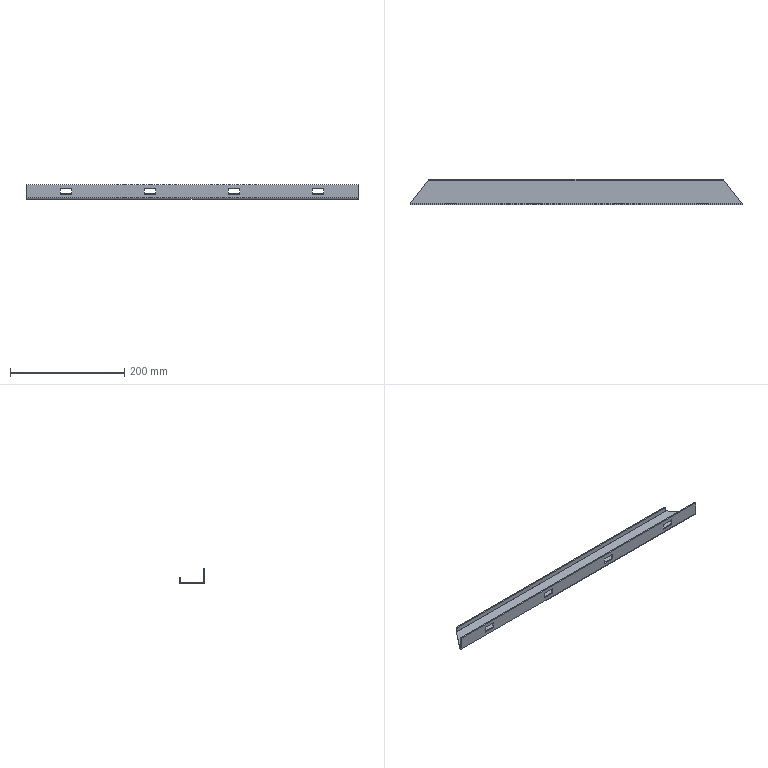Part | STEP file | Right Door Frame 4 | 1 solid | 36 faces | box 580 x 45 x 25 mm | volume 81646 mm3 | plane 32 | cylinder 4 | commonest cylinder face diameters 0.2 x2 4.2 x2
STEP:
#1=CARTESIAN_POINT('',(480.95,42.998,-6.375));
#2=VERTEX_POINT('',#1);
#3=CARTESIAN_POINT('',(480.95,43.,-6.375));
#4=VERTEX_POINT('',#3);
#5=CARTESIAN_POINT('',(480.95,40.9,-6.375));
#6=DIRECTION('',(0.,1.,0.));
#7=VECTOR('',#6,1000.);
#8=LINE('',#5,#7);
#9=EDGE_CURVE('',#2,#4,#8,.T.);
#10=ORIENTED_EDGE('',*,*,#9,.F.);
#11=CARTESIAN_POINT('',(480.95,40.9,-6.375));
#12=VERTEX_POINT('',#11);
#13=CARTESIAN_POINT('',(480.95,0.,-6.375));
#14=DIRECTION('',(0.,-1.,0.));
#15=VECTOR('',#14,1000.);
#16=LINE('',#13,#15);
#17=EDGE_CURVE('',#2,#12,#16,.T.);
#18=ORIENTED_EDGE('',*,*,#17,.T.);
#19=CARTESIAN_POINT('',(-33.05,40.9,-6.375));
#20=VERTEX_POINT('',#19);
#21=CARTESIAN_POINT('',(0.,40.9,-6.375));
#22=DIRECTION('',(-1.,0.,0.));
#23=VECTOR('',#22,1000.);
#24=LINE('',#21,#23);
#25=EDGE_CURVE('',#12,#20,#24,.T.);
#26=ORIENTED_EDGE('',*,*,#25,.T.);
#27=CARTESIAN_POINT('',(-33.05,42.998,-6.375));
#28=VERTEX_POINT('',#27);
#29=CARTESIAN_POINT('',(-33.05,0.,-6.375));
#30=DIRECTION('',(0.,1.,0.));
#31=VECTOR('',#30,1000.);
#32=LINE('',#29,#31);
#33=EDGE_CURVE('',#20,#28,#32,.T.);
#34=ORIENTED_EDGE('',*,*,#33,.T.);
#35=CARTESIAN_POINT('',(-33.05,43.,-6.375));
#36=VERTEX_POINT('',#35);
#37=CARTESIAN_POINT('',(-33.05,43.,-6.375));
#38=DIRECTION('',(0.,-1.,0.));
#39=VECTOR('',#38,1000.);
#40=LINE('',#37,#39);
#41=EDGE_CURVE('',#36,#28,#40,.T.);
#42=ORIENTED_EDGE('',*,*,#41,.F.);
#43=CARTESIAN_POINT('',(-66.05,0.2,-6.375));
#44=VERTEX_POINT('',#43);
#45=CARTESIAN_POINT('',(-33.05,43.,-6.375));
#46=DIRECTION('',(-0.6106,-0.7919,0.));
#47=VECTOR('',#46,1000.);
#48=LINE('',#45,#47);
#49=EDGE_CURVE('',#36,#44,#48,.T.);
#50=ORIENTED_EDGE('',*,*,#49,.T.);
#51=CARTESIAN_POINT('',(-66.05,0.1,-6.375));
#52=VERTEX_POINT('',#51);
#53=CARTESIAN_POINT('',(-66.05,43.,-6.375));
#54=DIRECTION('',(0.,-1.,0.));
#55=VECTOR('',#54,1000.);
#56=LINE('',#53,#55);
#57=EDGE_CURVE('',#44,#52,#56,.T.);
#58=ORIENTED_EDGE('',*,*,#57,.T.);
#59=CARTESIAN_POINT('',(513.95,0.1,-6.375));
#60=VERTEX_POINT('',#59);
#61=CARTESIAN_POINT('',(0.,0.1,-6.375));
#62=DIRECTION('',(1.,0.,0.));
#63=VECTOR('',#62,1000.);
#64=LINE('',#61,#63);
#65=EDGE_CURVE('',#52,#60,#64,.T.);
#66=ORIENTED_EDGE('',*,*,#65,.T.);
#67=CARTESIAN_POINT('',(513.95,0.2,-6.375));
#68=VERTEX_POINT('',#67);
#69=CARTESIAN_POINT('',(513.95,0.,-6.375));
#70=DIRECTION('',(0.,1.,0.));
#71=VECTOR('',#70,1000.);
#72=LINE('',#69,#71);
#73=EDGE_CURVE('',#60,#68,#72,.T.);
#74=ORIENTED_EDGE('',*,*,#73,.T.);
#75=CARTESIAN_POINT('',(513.95,0.2,-6.375));
#76=DIRECTION('',(-0.6106,0.7919,0.));
#77=VECTOR('',#76,1000.);
#78=LINE('',#75,#77);
#79=EDGE_CURVE('',#68,#4,#78,.T.);
#80=ORIENTED_EDGE('',*,*,#79,.T.);
#81=EDGE_LOOP('',(#10,#18,#26,#34,#42,#50,#58,#66,#74,#80));
#82=FACE_OUTER_BOUND('',#81,.T.);
#83=CARTESIAN_POINT('',(0.,0.,-6.375));
#84=DIRECTION('',(0.,0.,1.));
#85=DIRECTION('',(0.,-1.,0.));
#86=AXIS2_PLACEMENT_3D('',#83,#84,#85);
#87=PLANE('',#86);
#88=ADVANCED_FACE('',(#82),#87,.T.);
#89=CARTESIAN_POINT('',(480.95,43.,-6.275));
#90=VERTEX_POINT('',#89);
#91=CARTESIAN_POINT('',(480.95,40.9,-6.275));
#92=DIRECTION('',(-1.,0.,0.));
#93=DIRECTION('',(0.,0.,1.));
#94=AXIS2_PLACEMENT_3D('',#91,#92,#93);
#95=CIRCLE('',#94,2.1);
#96=EDGE_CURVE('',#90,#2,#95,.T.);
#97=ORIENTED_EDGE('',*,*,#96,.F.);
#98=CARTESIAN_POINT('',(480.95,43.,1.625));
#99=VERTEX_POINT('',#98);
#100=CARTESIAN_POINT('',(480.95,43.,-6.375));
#101=DIRECTION('',(0.,0.,-1.));
#102=VECTOR('',#101,1000.);
#103=LINE('',#100,#102);
#104=EDGE_CURVE('',#99,#90,#103,.T.);
#105=ORIENTED_EDGE('',*,*,#104,.F.);
#106=CARTESIAN_POINT('',(480.95,41.,1.625));
#107=VERTEX_POINT('',#106);
#108=CARTESIAN_POINT('',(480.95,43.,1.625));
#109=DIRECTION('',(0.,1.,0.));
#110=VECTOR('',#109,1000.);
#111=LINE('',#108,#110);
#112=EDGE_CURVE('',#107,#99,#111,.T.);
#113=ORIENTED_EDGE('',*,*,#112,.F.);
#114=CARTESIAN_POINT('',(480.95,41.,-6.275));
#115=VERTEX_POINT('',#114);
#116=CARTESIAN_POINT('',(480.95,41.,-6.375));
#117=DIRECTION('',(0.,0.,1.));
#118=VECTOR('',#117,1000.);
#119=LINE('',#116,#118);
#120=EDGE_CURVE('',#115,#107,#119,.T.);
#121=ORIENTED_EDGE('',*,*,#120,.F.);
#122=CARTESIAN_POINT('',(480.95,40.9,-6.275));
#123=DIRECTION('',(-1.,0.,0.));
#124=DIRECTION('',(0.,0.,1.));
#125=AXIS2_PLACEMENT_3D('',#122,#123,#124);
#126=CIRCLE('',#125,0.1);
#127=EDGE_CURVE('',#115,#12,#126,.T.);
#128=ORIENTED_EDGE('',*,*,#127,.T.);
#129=ORIENTED_EDGE('',*,*,#17,.F.);
#130=EDGE_LOOP('',(#97,#105,#113,#121,#128,#129));
#131=FACE_OUTER_BOUND('',#130,.T.);
#132=CARTESIAN_POINT('',(480.95,40.9,-6.275));
#133=DIRECTION('',(1.,0.,0.));
#134=DIRECTION('',(0.,0.,-1.));
#135=AXIS2_PLACEMENT_3D('',#132,#133,#134);
#136=PLANE('',#135);
#137=ADVANCED_FACE('',(#131),#136,.T.);
#138=CARTESIAN_POINT('',(513.95,0.2,-8.375));
#139=VERTEX_POINT('',#138);
#140=CARTESIAN_POINT('',(513.95,0.2,1.625));
#141=DIRECTION('',(0.,0.,1.));
#142=VECTOR('',#141,1000.);
#143=LINE('',#140,#142);
#144=EDGE_CURVE('',#139,#68,#143,.T.);
#145=ORIENTED_EDGE('',*,*,#144,.F.);
#146=CARTESIAN_POINT('',(480.95,43.,-8.375));
#147=VERTEX_POINT('',#146);
#148=CARTESIAN_POINT('',(513.95,0.2,-8.375));
#149=DIRECTION('',(0.6106,-0.7919,0.));
#150=VECTOR('',#149,1000.);
#151=LINE('',#148,#150);
#152=EDGE_CURVE('',#147,#139,#151,.T.);
#153=ORIENTED_EDGE('',*,*,#152,.F.);
#154=CARTESIAN_POINT('',(480.95,43.,1.625));
#155=DIRECTION('',(0.,0.,-1.));
#156=VECTOR('',#155,1000.);
#157=LINE('',#154,#156);
#158=EDGE_CURVE('',#4,#147,#157,.T.);
#159=ORIENTED_EDGE('',*,*,#158,.F.);
#160=ORIENTED_EDGE('',*,*,#79,.F.);
#161=EDGE_LOOP('',(#145,#153,#159,#160));
#162=FACE_OUTER_BOUND('',#161,.T.);
#163=CARTESIAN_POINT('',(513.95,0.2,1.625));
#164=DIRECTION('',(-0.7919,-0.6106,0.));
#165=DIRECTION('',(0.6106,-0.7919,0.));
#166=AXIS2_PLACEMENT_3D('',#163,#164,#165);
#167=PLANE('',#166);
#168=ADVANCED_FACE('',(#162),#167,.F.);
#169=CARTESIAN_POINT('',(513.95,0.,-6.275));
#170=VERTEX_POINT('',#169);
#171=CARTESIAN_POINT('',(513.95,0.1,-6.275));
#172=DIRECTION('',(-1.,0.,0.));
#173=DIRECTION('',(0.,-1.,0.));
#174=AXIS2_PLACEMENT_3D('',#171,#172,#173);
#175=CIRCLE('',#174,0.1);
#176=EDGE_CURVE('',#60,#170,#175,.T.);
#177=ORIENTED_EDGE('',*,*,#176,.F.);
#178=ORIENTED_EDGE('',*,*,#65,.F.);
#179=CARTESIAN_POINT('',(-66.05,0.,-6.275));
#180=VERTEX_POINT('',#179);
#181=CARTESIAN_POINT('',(-66.05,0.1,-6.275));
#182=DIRECTION('',(-1.,0.,0.));
#183=DIRECTION('',(0.,-1.,0.));
#184=AXIS2_PLACEMENT_3D('',#181,#182,#183);
#185=CIRCLE('',#184,0.1);
#186=EDGE_CURVE('',#52,#180,#185,.T.);
#187=ORIENTED_EDGE('',*,*,#186,.T.);
#188=CARTESIAN_POINT('',(-66.05,0.,-6.275));
#189=DIRECTION('',(-1.,0.,0.));
#190=VECTOR('',#189,1000.);
#191=LINE('',#188,#190);
#192=EDGE_CURVE('',#170,#180,#191,.T.);
#193=ORIENTED_EDGE('',*,*,#192,.F.);
#194=EDGE_LOOP('',(#177,#178,#187,#193));
#195=FACE_OUTER_BOUND('',#194,.T.);
#196=CARTESIAN_POINT('',(-66.05,0.1,-6.275));
#197=DIRECTION('',(-1.,0.,0.));
#198=DIRECTION('',(0.,-1.,0.));
#199=AXIS2_PLACEMENT_3D('',#196,#197,#198);
#200=CYLINDRICAL_SURFACE('',#199,0.1);
#201=ADVANCED_FACE('',(#195),#200,.F.);
#202=CARTESIAN_POINT('',(-33.05,43.,-8.375));
#203=VERTEX_POINT('',#202);
#204=CARTESIAN_POINT('',(-33.05,43.,1.625));
#205=DIRECTION('',(0.,0.,1.));
#206=VECTOR('',#205,1000.);
#207=LINE('',#204,#206);
#208=EDGE_CURVE('',#203,#36,#207,.T.);
#209=ORIENTED_EDGE('',*,*,#208,.F.);
#210=CARTESIAN_POINT('',(-66.05,0.2,-8.375));
#211=VERTEX_POINT('',#210);
#212=CARTESIAN_POINT('',(-66.05,0.2,-8.375));
#213=DIRECTION('',(0.6106,0.7919,0.));
#214=VECTOR('',#213,1000.);
#215=LINE('',#212,#214);
#216=EDGE_CURVE('',#211,#203,#215,.T.);
#217=ORIENTED_EDGE('',*,*,#216,.F.);
#218=CARTESIAN_POINT('',(-66.05,0.2,1.625));
#219=DIRECTION('',(0.,0.,-1.));
#220=VECTOR('',#219,1000.);
#221=LINE('',#218,#220);
#222=EDGE_CURVE('',#44,#211,#221,.T.);
#223=ORIENTED_EDGE('',*,*,#222,.F.);
#224=ORIENTED_EDGE('',*,*,#49,.F.);
#225=EDGE_LOOP('',(#209,#217,#223,#224));
#226=FACE_OUTER_BOUND('',#225,.T.);
#227=CARTESIAN_POINT('',(-66.05,0.2,1.625));
#228=DIRECTION('',(0.7919,-0.6106,0.));
#229=DIRECTION('',(0.6106,0.7919,0.));
#230=AXIS2_PLACEMENT_3D('',#227,#228,#229);
#231=PLANE('',#230);
#232=ADVANCED_FACE('',(#226),#231,.F.);
#233=ORIENTED_EDGE('',*,*,#33,.F.);
#234=CARTESIAN_POINT('',(-33.05,41.,-6.275));
#235=VERTEX_POINT('',#234);
#236=CARTESIAN_POINT('',(-33.05,40.9,-6.275));
#237=DIRECTION('',(-1.,0.,0.));
#238=DIRECTION('',(0.,0.,1.));
#239=AXIS2_PLACEMENT_3D('',#236,#237,#238);
#240=CIRCLE('',#239,0.1);
#241=EDGE_CURVE('',#235,#20,#240,.T.);
#242=ORIENTED_EDGE('',*,*,#241,.F.);
#243=CARTESIAN_POINT('',(-33.05,41.,1.625));
#244=VERTEX_POINT('',#243);
#245=CARTESIAN_POINT('',(-33.05,41.,1.625));
#246=DIRECTION('',(0.,0.,-1.));
#247=VECTOR('',#246,1000.);
#248=LINE('',#245,#247);
#249=EDGE_CURVE('',#244,#235,#248,.T.);
#250=ORIENTED_EDGE('',*,*,#249,.F.);
#251=CARTESIAN_POINT('',(-33.05,43.,1.625));
#252=VERTEX_POINT('',#251);
#253=CARTESIAN_POINT('',(-33.05,43.,1.625));
#254=DIRECTION('',(0.,-1.,0.));
#255=VECTOR('',#254,1000.);
#256=LINE('',#253,#255);
#257=EDGE_CURVE('',#252,#244,#256,.T.);
#258=ORIENTED_EDGE('',*,*,#257,.F.);
#259=CARTESIAN_POINT('',(-33.05,43.,-6.275));
#260=VERTEX_POINT('',#259);
#261=CARTESIAN_POINT('',(-33.05,43.,1.625));
#262=DIRECTION('',(0.,0.,1.));
#263=VECTOR('',#262,1000.);
#264=LINE('',#261,#263);
#265=EDGE_CURVE('',#260,#252,#264,.T.);
#266=ORIENTED_EDGE('',*,*,#265,.F.);
#267=CARTESIAN_POINT('',(-33.05,40.9,-6.275));
#268=DIRECTION('',(1.,0.,0.));
#269=DIRECTION('',(0.,0.,1.));
#270=AXIS2_PLACEMENT_3D('',#267,#268,#269);
#271=CIRCLE('',#270,2.1);
#272=EDGE_CURVE('',#28,#260,#271,.T.);
#273=ORIENTED_EDGE('',*,*,#272,.F.);
#274=EDGE_LOOP('',(#233,#242,#250,#258,#266,#273));
#275=FACE_OUTER_BOUND('',#274,.T.);
#276=CARTESIAN_POINT('',(-33.05,40.9,-6.275));
#277=DIRECTION('',(1.,0.,0.));
#278=DIRECTION('',(0.,0.,-1.));
#279=AXIS2_PLACEMENT_3D('',#276,#277,#278);
#280=PLANE('',#279);
#281=ADVANCED_FACE('',(#275),#280,.F.);
#282=ORIENTED_EDGE('',*,*,#127,.F.);
#283=CARTESIAN_POINT('',(-33.05,41.,-6.275));
#284=DIRECTION('',(1.,0.,0.));
#285=VECTOR('',#284,1000.);
#286=LINE('',#283,#285);
#287=EDGE_CURVE('',#235,#115,#286,.T.);
#288=ORIENTED_EDGE('',*,*,#287,.F.);
#289=ORIENTED_EDGE('',*,*,#241,.T.);
#290=ORIENTED_EDGE('',*,*,#25,.F.);
#291=EDGE_LOOP('',(#282,#288,#289,#290));
#292=FACE_OUTER_BOUND('',#291,.T.);
#293=CARTESIAN_POINT('',(-33.05,40.9,-6.275));
#294=DIRECTION('',(-1.,0.,0.));
#295=DIRECTION('',(0.,0.,1.));
#296=AXIS2_PLACEMENT_3D('',#293,#294,#295);
#297=CYLINDRICAL_SURFACE('',#296,0.1);
#298=ADVANCED_FACE('',(#292),#297,.F.);
#299=ORIENTED_EDGE('',*,*,#144,.T.);
#300=ORIENTED_EDGE('',*,*,#73,.F.);
#301=ORIENTED_EDGE('',*,*,#176,.T.);
#302=CARTESIAN_POINT('',(513.95,0.,16.625));
#303=VERTEX_POINT('',#302);
#304=CARTESIAN_POINT('',(513.95,0.,0.));
#305=DIRECTION('',(0.,0.,-1.));
#306=VECTOR('',#305,1000.);
#307=LINE('',#304,#306);
#308=EDGE_CURVE('',#303,#170,#307,.T.);
#309=ORIENTED_EDGE('',*,*,#308,.F.);
#310=CARTESIAN_POINT('',(513.95,-2.,16.625));
#311=VERTEX_POINT('',#310);
#312=CARTESIAN_POINT('',(513.95,-2.,16.625));
#313=DIRECTION('',(0.,1.,0.));
#314=VECTOR('',#313,1000.);
#315=LINE('',#312,#314);
#316=EDGE_CURVE('',#311,#303,#315,.T.);
#317=ORIENTED_EDGE('',*,*,#316,.F.);
#318=CARTESIAN_POINT('',(513.95,-2.,-6.275));
#319=VERTEX_POINT('',#318);
#320=CARTESIAN_POINT('',(513.95,-2.,-8.375));
#321=DIRECTION('',(0.,0.,-1.));
#322=VECTOR('',#321,1000.);
#323=LINE('',#320,#322);
#324=EDGE_CURVE('',#311,#319,#323,.T.);
#325=ORIENTED_EDGE('',*,*,#324,.T.);
#326=CARTESIAN_POINT('',(513.95,0.1,-8.375));
#327=VERTEX_POINT('',#326);
#328=CARTESIAN_POINT('',(513.95,0.1,-6.275));
#329=DIRECTION('',(1.,0.,0.));
#330=DIRECTION('',(0.,-1.,0.));
#331=AXIS2_PLACEMENT_3D('',#328,#329,#330);
#332=CIRCLE('',#331,2.1);
#333=EDGE_CURVE('',#319,#327,#332,.T.);
#334=ORIENTED_EDGE('',*,*,#333,.T.);
#335=CARTESIAN_POINT('',(513.95,0.,-8.375));
#336=DIRECTION('',(0.,-1.,0.));
#337=VECTOR('',#336,1000.);
#338=LINE('',#335,#337);
#339=EDGE_CURVE('',#139,#327,#338,.T.);
#340=ORIENTED_EDGE('',*,*,#339,.F.);
#341=EDGE_LOOP('',(#299,#300,#301,#309,#317,#325,#334,#340));
#342=FACE_OUTER_BOUND('',#341,.T.);
#343=CARTESIAN_POINT('',(513.95,0.,-8.375));
#344=DIRECTION('',(-1.,0.,0.));
#345=DIRECTION('',(0.,0.,1.));
#346=AXIS2_PLACEMENT_3D('',#343,#344,#345);
#347=PLANE('',#346);
#348=ADVANCED_FACE('',(#342),#347,.F.);
#349=CARTESIAN_POINT('',(480.95,40.9,-8.375));
#350=VERTEX_POINT('',#349);
#351=CARTESIAN_POINT('',(-33.05,40.9,-8.375));
#352=VERTEX_POINT('',#351);
#353=CARTESIAN_POINT('',(0.,40.9,-8.375));
#354=DIRECTION('',(-1.,0.,0.));
#355=VECTOR('',#354,1000.);
#356=LINE('',#353,#355);
#357=EDGE_CURVE('',#350,#352,#356,.T.);
#358=ORIENTED_EDGE('',*,*,#357,.F.);
#359=CARTESIAN_POINT('',(480.95,0.,-8.375));
#360=DIRECTION('',(0.,-1.,0.));
#361=VECTOR('',#360,1000.);
#362=LINE('',#359,#361);
#363=EDGE_CURVE('',#147,#350,#362,.T.);
#364=ORIENTED_EDGE('',*,*,#363,.F.);
#365=ORIENTED_EDGE('',*,*,#152,.T.);
#366=ORIENTED_EDGE('',*,*,#339,.T.);
#367=CARTESIAN_POINT('',(-66.05,0.1,-8.375));
#368=VERTEX_POINT('',#367);
#369=CARTESIAN_POINT('',(0.,0.1,-8.375));
#370=DIRECTION('',(1.,0.,0.));
#371=VECTOR('',#370,1000.);
#372=LINE('',#369,#371);
#373=EDGE_CURVE('',#368,#327,#372,.T.);
#374=ORIENTED_EDGE('',*,*,#373,.F.);
#375=CARTESIAN_POINT('',(-66.05,0.,-8.375));
#376=DIRECTION('',(0.,-1.,0.));
#377=VECTOR('',#376,1000.);
#378=LINE('',#375,#377);
#379=EDGE_CURVE('',#211,#368,#378,.T.);
#380=ORIENTED_EDGE('',*,*,#379,.F.);
#381=ORIENTED_EDGE('',*,*,#216,.T.);
#382=CARTESIAN_POINT('',(-33.05,0.,-8.375));
#383=DIRECTION('',(0.,1.,0.));
#384=VECTOR('',#383,1000.);
#385=LINE('',#382,#384);
#386=EDGE_CURVE('',#352,#203,#385,.T.);
#387=ORIENTED_EDGE('',*,*,#386,.F.);
#388=EDGE_LOOP('',(#358,#364,#365,#366,#374,#380,#381,#387));
#389=FACE_OUTER_BOUND('',#388,.T.);
#390=CARTESIAN_POINT('',(0.,0.,-8.375));
#391=DIRECTION('',(0.,0.,1.));
#392=DIRECTION('',(0.,-1.,0.));
#393=AXIS2_PLACEMENT_3D('',#390,#391,#392);
#394=PLANE('',#393);
#395=ADVANCED_FACE('',(#389),#394,.F.);
#396=ORIENTED_EDGE('',*,*,#9,.T.);
#397=ORIENTED_EDGE('',*,*,#158,.T.);
#398=ORIENTED_EDGE('',*,*,#363,.T.);
#399=CARTESIAN_POINT('',(480.95,40.9,-6.275));
#400=DIRECTION('',(1.,0.,0.));
#401=DIRECTION('',(0.,0.,1.));
#402=AXIS2_PLACEMENT_3D('',#399,#400,#401);
#403=CIRCLE('',#402,2.1);
#404=EDGE_CURVE('',#350,#2,#403,.T.);
#405=ORIENTED_EDGE('',*,*,#404,.T.);
#406=EDGE_LOOP('',(#396,#397,#398,#405));
#407=FACE_OUTER_BOUND('',#406,.T.);
#408=CARTESIAN_POINT('',(480.95,40.9,-6.375));
#409=DIRECTION('',(-1.,0.,0.));
#410=DIRECTION('',(0.,0.,1.));
#411=AXIS2_PLACEMENT_3D('',#408,#409,#410);
#412=PLANE('',#411);
#413=ADVANCED_FACE('',(#407),#412,.T.);
#414=CARTESIAN_POINT('',(-66.05,0.,16.625));
#415=VERTEX_POINT('',#414);
#416=CARTESIAN_POINT('',(-66.05,0.,0.));
#417=DIRECTION('',(0.,0.,1.));
#418=VECTOR('',#417,1000.);
#419=LINE('',#416,#418);
#420=EDGE_CURVE('',#180,#415,#419,.T.);
#421=ORIENTED_EDGE('',*,*,#420,.T.);
#422=CARTESIAN_POINT('',(0.,0.,16.625));
#423=DIRECTION('',(1.,0.,0.));
#424=VECTOR('',#423,1000.);
#425=LINE('',#422,#424);
#426=EDGE_CURVE('',#415,#303,#425,.T.);
#427=ORIENTED_EDGE('',*,*,#426,.T.);
#428=ORIENTED_EDGE('',*,*,#308,.T.);
#429=ORIENTED_EDGE('',*,*,#192,.T.);
#430=EDGE_LOOP('',(#421,#427,#428,#429));
#431=FACE_OUTER_BOUND('',#430,.T.);
#432=CARTESIAN_POINT('',(13.95,0.,-0.1248));
#433=VERTEX_POINT('',#432);
#434=CARTESIAN_POINT('',(13.95,0.,9.875));
#435=VERTEX_POINT('',#434);
#436=CARTESIAN_POINT('',(13.95,0.,0.));
#437=DIRECTION('',(0.,0.,1.));
#438=VECTOR('',#437,1000.);
#439=LINE('',#436,#438);
#440=EDGE_CURVE('',#433,#435,#439,.T.);
#441=ORIENTED_EDGE('',*,*,#440,.T.);
#442=CARTESIAN_POINT('',(-6.05,0.,9.875));
#443=VERTEX_POINT('',#442);
#444=CARTESIAN_POINT('',(0.,0.,9.875));
#445=DIRECTION('',(-1.,0.,0.));
#446=VECTOR('',#445,1000.);
#447=LINE('',#444,#446);
#448=EDGE_CURVE('',#435,#443,#447,.T.);
#449=ORIENTED_EDGE('',*,*,#448,.T.);
#450=CARTESIAN_POINT('',(-6.05,0.,-0.1248));
#451=VERTEX_POINT('',#450);
#452=CARTESIAN_POINT('',(-6.05,0.,0.));
#453=DIRECTION('',(0.,0.,-1.));
#454=VECTOR('',#453,1000.);
#455=LINE('',#452,#454);
#456=EDGE_CURVE('',#443,#451,#455,.T.);
#457=ORIENTED_EDGE('',*,*,#456,.T.);
#458=CARTESIAN_POINT('',(0.,0.,-0.1248));
#459=DIRECTION('',(1.,0.,0.));
#460=VECTOR('',#459,1000.);
#461=LINE('',#458,#460);
#462=EDGE_CURVE('',#451,#433,#461,.T.);
#463=ORIENTED_EDGE('',*,*,#462,.T.);
#464=EDGE_LOOP('',(#441,#449,#457,#463));
#465=FACE_BOUND('',#464,.T.);
#466=CARTESIAN_POINT('',(160.617,0.,-0.1248));
#467=VERTEX_POINT('',#466);
#468=CARTESIAN_POINT('',(160.617,0.,9.875));
#469=VERTEX_POINT('',#468);
#470=CARTESIAN_POINT('',(160.617,0.,0.));
#471=DIRECTION('',(0.,0.,1.));
#472=VECTOR('',#471,1000.);
#473=LINE('',#470,#472);
#474=EDGE_CURVE('',#467,#469,#473,.T.);
#475=ORIENTED_EDGE('',*,*,#474,.T.);
#476=CARTESIAN_POINT('',(140.617,0.,9.875));
#477=VERTEX_POINT('',#476);
#478=CARTESIAN_POINT('',(0.,0.,9.875));
#479=DIRECTION('',(-1.,0.,0.));
#480=VECTOR('',#479,1000.);
#481=LINE('',#478,#480);
#482=EDGE_CURVE('',#469,#477,#481,.T.);
#483=ORIENTED_EDGE('',*,*,#482,.T.);
#484=CARTESIAN_POINT('',(140.617,0.,-0.1248));
#485=VERTEX_POINT('',#484);
#486=CARTESIAN_POINT('',(140.617,0.,0.));
#487=DIRECTION('',(0.,0.,-1.));
#488=VECTOR('',#487,1000.);
#489=LINE('',#486,#488);
#490=EDGE_CURVE('',#477,#485,#489,.T.);
#491=ORIENTED_EDGE('',*,*,#490,.T.);
#492=CARTESIAN_POINT('',(0.,0.,-0.1248));
#493=DIRECTION('',(1.,0.,0.));
#494=VECTOR('',#493,1000.);
#495=LINE('',#492,#494);
#496=EDGE_CURVE('',#485,#467,#495,.T.);
#497=ORIENTED_EDGE('',*,*,#496,.T.);
#498=EDGE_LOOP('',(#475,#483,#491,#497));
#499=FACE_BOUND('',#498,.T.);
#500=CARTESIAN_POINT('',(307.283,0.,-0.1248));
#501=VERTEX_POINT('',#500);
#502=CARTESIAN_POINT('',(307.283,0.,9.875));
#503=VERTEX_POINT('',#502);
#504=CARTESIAN_POINT('',(307.283,0.,0.));
#505=DIRECTION('',(0.,0.,1.));
#506=VECTOR('',#505,1000.);
#507=LINE('',#504,#506);
#508=EDGE_CURVE('',#501,#503,#507,.T.);
#509=ORIENTED_EDGE('',*,*,#508,.T.);
#510=CARTESIAN_POINT('',(287.283,0.,9.875));
#511=VERTEX_POINT('',#510);
#512=CARTESIAN_POINT('',(0.,0.,9.875));
#513=DIRECTION('',(-1.,0.,0.));
#514=VECTOR('',#513,1000.);
#515=LINE('',#512,#514);
#516=EDGE_CURVE('',#503,#511,#515,.T.);
#517=ORIENTED_EDGE('',*,*,#516,.T.);
#518=CARTESIAN_POINT('',(287.283,0.,-0.1248));
#519=VERTEX_POINT('',#518);
#520=CARTESIAN_POINT('',(287.283,0.,0.));
#521=DIRECTION('',(0.,0.,-1.));
#522=VECTOR('',#521,1000.);
#523=LINE('',#520,#522);
#524=EDGE_CURVE('',#511,#519,#523,.T.);
#525=ORIENTED_EDGE('',*,*,#524,.T.);
#526=CARTESIAN_POINT('',(0.,0.,-0.1248));
#527=DIRECTION('',(1.,0.,0.));
#528=VECTOR('',#527,1000.);
#529=LINE('',#526,#528);
#530=EDGE_CURVE('',#519,#501,#529,.T.);
#531=ORIENTED_EDGE('',*,*,#530,.T.);
#532=EDGE_LOOP('',(#509,#517,#525,#531));
#533=FACE_BOUND('',#532,.T.);
#534=CARTESIAN_POINT('',(453.95,0.,-0.1248));
#535=VERTEX_POINT('',#534);
#536=CARTESIAN_POINT('',(453.95,0.,9.875));
#537=VERTEX_POINT('',#536);
#538=CARTESIAN_POINT('',(453.95,0.,0.));
#539=DIRECTION('',(0.,0.,1.));
#540=VECTOR('',#539,1000.);
#541=LINE('',#538,#540);
#542=EDGE_CURVE('',#535,#537,#541,.T.);
#543=ORIENTED_EDGE('',*,*,#542,.T.);
#544=CARTESIAN_POINT('',(433.95,0.,9.875));
#545=VERTEX_POINT('',#544);
#546=CARTESIAN_POINT('',(0.,0.,9.875));
#547=DIRECTION('',(-1.,0.,0.));
#548=VECTOR('',#547,1000.);
#549=LINE('',#546,#548);
#550=EDGE_CURVE('',#537,#545,#549,.T.);
#551=ORIENTED_EDGE('',*,*,#550,.T.);
#552=CARTESIAN_POINT('',(433.95,0.,-0.1248));
#553=VERTEX_POINT('',#552);
#554=CARTESIAN_POINT('',(433.95,0.,0.));
#555=DIRECTION('',(0.,0.,-1.));
#556=VECTOR('',#555,1000.);
#557=LINE('',#554,#556);
#558=EDGE_CURVE('',#545,#553,#557,.T.);
#559=ORIENTED_EDGE('',*,*,#558,.T.);
#560=CARTESIAN_POINT('',(0.,0.,-0.1248));
#561=DIRECTION('',(1.,0.,0.));
#562=VECTOR('',#561,1000.);
#563=LINE('',#560,#562);
#564=EDGE_CURVE('',#553,#535,#563,.T.);
#565=ORIENTED_EDGE('',*,*,#564,.T.);
#566=EDGE_LOOP('',(#543,#551,#559,#565));
#567=FACE_BOUND('',#566,.T.);
#568=CARTESIAN_POINT('',(0.,0.,0.));
#569=DIRECTION('',(0.,1.,0.));
#570=DIRECTION('',(0.,0.,1.));
#571=AXIS2_PLACEMENT_3D('',#568,#569,#570);
#572=PLANE('',#571);
#573=ADVANCED_FACE('',(#431,#465,#499,#533,#567),#572,.T.);
#574=ORIENTED_EDGE('',*,*,#386,.T.);
#575=ORIENTED_EDGE('',*,*,#208,.T.);
#576=ORIENTED_EDGE('',*,*,#41,.T.);
#577=CARTESIAN_POINT('',(-33.05,40.9,-6.275));
#578=DIRECTION('',(-1.,0.,0.));
#579=DIRECTION('',(0.,0.,1.));
#580=AXIS2_PLACEMENT_3D('',#577,#578,#579);
#581=CIRCLE('',#580,2.1);
#582=EDGE_CURVE('',#28,#352,#581,.T.);
#583=ORIENTED_EDGE('',*,*,#582,.T.);
#584=EDGE_LOOP('',(#574,#575,#576,#583));
#585=FACE_OUTER_BOUND('',#584,.T.);
#586=CARTESIAN_POINT('',(-33.05,43.,-6.375));
#587=DIRECTION('',(1.,0.,0.));
#588=DIRECTION('',(0.,0.,-1.));
#589=AXIS2_PLACEMENT_3D('',#586,#587,#588);
#590=PLANE('',#589);
#591=ADVANCED_FACE('',(#585),#590,.T.);
#592=ORIENTED_EDGE('',*,*,#222,.T.);
#593=ORIENTED_EDGE('',*,*,#379,.T.);
#594=CARTESIAN_POINT('',(-66.05,-2.,-6.275));
#595=VERTEX_POINT('',#594);
#596=CARTESIAN_POINT('',(-66.05,0.1,-6.275));
#597=DIRECTION('',(1.,0.,0.));
#598=DIRECTION('',(0.,-1.,0.));
#599=AXIS2_PLACEMENT_3D('',#596,#597,#598);
#600=CIRCLE('',#599,2.1);
#601=EDGE_CURVE('',#595,#368,#600,.T.);
#602=ORIENTED_EDGE('',*,*,#601,.F.);
#603=CARTESIAN_POINT('',(-66.05,-2.,16.625));
#604=VERTEX_POINT('',#603);
#605=CARTESIAN_POINT('',(-66.05,-2.,-8.375));
#606=DIRECTION('',(0.,0.,1.));
#607=VECTOR('',#606,1000.);
#608=LINE('',#605,#607);
#609=EDGE_CURVE('',#595,#604,#608,.T.);
#610=ORIENTED_EDGE('',*,*,#609,.T.);
#611=CARTESIAN_POINT('',(-66.05,-2.,16.625));
#612=DIRECTION('',(0.,-1.,0.));
#613=VECTOR('',#612,1000.);
#614=LINE('',#611,#613);
#615=EDGE_CURVE('',#415,#604,#614,.T.);
#616=ORIENTED_EDGE('',*,*,#615,.F.);
#617=ORIENTED_EDGE('',*,*,#420,.F.);
#618=ORIENTED_EDGE('',*,*,#186,.F.);
#619=ORIENTED_EDGE('',*,*,#57,.F.);
#620=EDGE_LOOP('',(#592,#593,#602,#610,#616,#617,#618,#619));
#621=FACE_OUTER_BOUND('',#620,.T.);
#622=CARTESIAN_POINT('',(-66.05,43.,-8.375));
#623=DIRECTION('',(1.,0.,0.));
#624=DIRECTION('',(0.,0.,-1.));
#625=AXIS2_PLACEMENT_3D('',#622,#623,#624);
#626=PLANE('',#625);
#627=ADVANCED_FACE('',(#621),#626,.F.);
#628=ORIENTED_EDGE('',*,*,#120,.T.);
#629=CARTESIAN_POINT('',(0.,41.,1.625));
#630=DIRECTION('',(-1.,0.,0.));
#631=VECTOR('',#630,1000.);
#632=LINE('',#629,#631);
#633=EDGE_CURVE('',#107,#244,#632,.T.);
#634=ORIENTED_EDGE('',*,*,#633,.T.);
#635=ORIENTED_EDGE('',*,*,#249,.T.);
#636=ORIENTED_EDGE('',*,*,#287,.T.);
#637=EDGE_LOOP('',(#628,#634,#635,#636));
#638=FACE_OUTER_BOUND('',#637,.T.);
#639=CARTESIAN_POINT('',(0.,41.,0.));
#640=DIRECTION('',(0.,-1.,0.));
#641=DIRECTION('',(0.,0.,-1.));
#642=AXIS2_PLACEMENT_3D('',#639,#640,#641);
#643=PLANE('',#642);
#644=ADVANCED_FACE('',(#638),#643,.T.);
#645=ORIENTED_EDGE('',*,*,#265,.T.);
#646=CARTESIAN_POINT('',(0.,43.,1.625));
#647=DIRECTION('',(-1.,0.,0.));
#648=VECTOR('',#647,1000.);
#649=LINE('',#646,#648);
#650=EDGE_CURVE('',#99,#252,#649,.T.);
#651=ORIENTED_EDGE('',*,*,#650,.F.);
#652=ORIENTED_EDGE('',*,*,#104,.T.);
#653=CARTESIAN_POINT('',(0.,43.,-6.275));
#654=DIRECTION('',(1.,0.,0.));
#655=VECTOR('',#654,1000.);
#656=LINE('',#653,#655);
#657=EDGE_CURVE('',#260,#90,#656,.T.);
#658=ORIENTED_EDGE('',*,*,#657,.F.);
#659=EDGE_LOOP('',(#645,#651,#652,#658));
#660=FACE_OUTER_BOUND('',#659,.T.);
#661=CARTESIAN_POINT('',(0.,43.,0.));
#662=DIRECTION('',(0.,-1.,0.));
#663=DIRECTION('',(0.,0.,-1.));
#664=AXIS2_PLACEMENT_3D('',#661,#662,#663);
#665=PLANE('',#664);
#666=ADVANCED_FACE('',(#660),#665,.F.);
#667=ORIENTED_EDGE('',*,*,#112,.T.);
#668=ORIENTED_EDGE('',*,*,#650,.T.);
#669=ORIENTED_EDGE('',*,*,#257,.T.);
#670=ORIENTED_EDGE('',*,*,#633,.F.);
#671=EDGE_LOOP('',(#667,#668,#669,#670));
#672=FACE_OUTER_BOUND('',#671,.T.);
#673=CARTESIAN_POINT('',(480.95,43.,1.625));
#674=DIRECTION('',(0.,0.,-1.));
#675=DIRECTION('',(0.,1.,0.));
#676=AXIS2_PLACEMENT_3D('',#673,#674,#675);
#677=PLANE('',#676);
#678=ADVANCED_FACE('',(#672),#677,.F.);
#679=ORIENTED_EDGE('',*,*,#96,.T.);
#680=ORIENTED_EDGE('',*,*,#404,.F.);
#681=ORIENTED_EDGE('',*,*,#357,.T.);
#682=ORIENTED_EDGE('',*,*,#582,.F.);
#683=ORIENTED_EDGE('',*,*,#272,.T.);
#684=ORIENTED_EDGE('',*,*,#657,.T.);
#685=EDGE_LOOP('',(#679,#680,#681,#682,#683,#684));
#686=FACE_OUTER_BOUND('',#685,.T.);
#687=CARTESIAN_POINT('',(-33.05,40.9,-6.275));
#688=DIRECTION('',(-1.,0.,0.));
#689=DIRECTION('',(0.,0.,1.));
#690=AXIS2_PLACEMENT_3D('',#687,#688,#689);
#691=CYLINDRICAL_SURFACE('',#690,2.1);
#692=ADVANCED_FACE('',(#686),#691,.T.);
#693=ORIENTED_EDGE('',*,*,#373,.T.);
#694=ORIENTED_EDGE('',*,*,#333,.F.);
#695=CARTESIAN_POINT('',(-66.05,-2.,-6.275));
#696=DIRECTION('',(-1.,0.,0.));
#697=VECTOR('',#696,1000.);
#698=LINE('',#695,#697);
#699=EDGE_CURVE('',#319,#595,#698,.T.);
#700=ORIENTED_EDGE('',*,*,#699,.T.);
#701=ORIENTED_EDGE('',*,*,#601,.T.);
#702=EDGE_LOOP('',(#693,#694,#700,#701));
#703=FACE_OUTER_BOUND('',#702,.T.);
#704=CARTESIAN_POINT('',(-66.05,0.1,-6.275));
#705=DIRECTION('',(-1.,0.,0.));
#706=DIRECTION('',(0.,-1.,0.));
#707=AXIS2_PLACEMENT_3D('',#704,#705,#706);
#708=CYLINDRICAL_SURFACE('',#707,2.1);
#709=ADVANCED_FACE('',(#703),#708,.T.);
#710=CARTESIAN_POINT('',(-66.05,-2.,16.625));
#711=DIRECTION('',(1.,0.,0.));
#712=VECTOR('',#711,1000.);
#713=LINE('',#710,#712);
#714=EDGE_CURVE('',#604,#311,#713,.T.);
#715=ORIENTED_EDGE('',*,*,#714,.T.);
#716=ORIENTED_EDGE('',*,*,#316,.T.);
#717=ORIENTED_EDGE('',*,*,#426,.F.);
#718=ORIENTED_EDGE('',*,*,#615,.T.);
#719=EDGE_LOOP('',(#715,#716,#717,#718));
#720=FACE_OUTER_BOUND('',#719,.T.);
#721=CARTESIAN_POINT('',(-66.05,-2.,16.625));
#722=DIRECTION('',(0.,0.,1.));
#723=DIRECTION('',(1.,0.,0.));
#724=AXIS2_PLACEMENT_3D('',#721,#722,#723);
#725=PLANE('',#724);
#726=ADVANCED_FACE('',(#720),#725,.T.);
#727=CARTESIAN_POINT('',(13.95,-2.,9.875));
#728=VERTEX_POINT('',#727);
#729=CARTESIAN_POINT('',(13.95,8.,9.875));
#730=DIRECTION('',(0.,1.,0.));
#731=VECTOR('',#730,1000.);
#732=LINE('',#729,#731);
#733=EDGE_CURVE('',#728,#435,#732,.T.);
#734=ORIENTED_EDGE('',*,*,#733,.F.);
#735=CARTESIAN_POINT('',(-6.05,-2.,9.875));
#736=VERTEX_POINT('',#735);
#737=CARTESIAN_POINT('',(-6.05,-2.,9.875));
#738=DIRECTION('',(1.,0.,0.));
#739=VECTOR('',#738,1000.);
#740=LINE('',#737,#739);
#741=EDGE_CURVE('',#736,#728,#740,.T.);
#742=ORIENTED_EDGE('',*,*,#741,.F.);
#743=CARTESIAN_POINT('',(-6.05,8.,9.875));
#744=DIRECTION('',(0.,-1.,0.));
#745=VECTOR('',#744,1000.);
#746=LINE('',#743,#745);
#747=EDGE_CURVE('',#443,#736,#746,.T.);
#748=ORIENTED_EDGE('',*,*,#747,.F.);
#749=ORIENTED_EDGE('',*,*,#448,.F.);
#750=EDGE_LOOP('',(#734,#742,#748,#749));
#751=FACE_OUTER_BOUND('',#750,.T.);
#752=CARTESIAN_POINT('',(-6.05,8.,9.875));
#753=DIRECTION('',(0.,0.,1.));
#754=DIRECTION('',(1.,0.,0.));
#755=AXIS2_PLACEMENT_3D('',#752,#753,#754);
#756=PLANE('',#755);
#757=ADVANCED_FACE('',(#751),#756,.F.);
#758=CARTESIAN_POINT('',(13.95,-2.,-0.1248));
#759=VERTEX_POINT('',#758);
#760=CARTESIAN_POINT('',(13.95,8.,-0.1248));
#761=DIRECTION('',(0.,1.,0.));
#762=VECTOR('',#761,1000.);
#763=LINE('',#760,#762);
#764=EDGE_CURVE('',#759,#433,#763,.T.);
#765=ORIENTED_EDGE('',*,*,#764,.F.);
#766=CARTESIAN_POINT('',(13.95,-2.,9.875));
#767=DIRECTION('',(0.,0.,-1.));
#768=VECTOR('',#767,1000.);
#769=LINE('',#766,#768);
#770=EDGE_CURVE('',#728,#759,#769,.T.);
#771=ORIENTED_EDGE('',*,*,#770,.F.);
#772=ORIENTED_EDGE('',*,*,#733,.T.);
#773=ORIENTED_EDGE('',*,*,#440,.F.);
#774=EDGE_LOOP('',(#765,#771,#772,#773));
#775=FACE_OUTER_BOUND('',#774,.T.);
#776=CARTESIAN_POINT('',(13.95,8.,9.875));
#777=DIRECTION('',(1.,0.,0.));
#778=DIRECTION('',(0.,0.,-1.));
#779=AXIS2_PLACEMENT_3D('',#776,#777,#778);
#780=PLANE('',#779);
#781=ADVANCED_FACE('',(#775),#780,.F.);
#782=CARTESIAN_POINT('',(-6.05,-2.,-0.1248));
#783=VERTEX_POINT('',#782);
#784=CARTESIAN_POINT('',(-6.05,8.,-0.1248));
#785=DIRECTION('',(0.,1.,0.));
#786=VECTOR('',#785,1000.);
#787=LINE('',#784,#786);
#788=EDGE_CURVE('',#783,#451,#787,.T.);
#789=ORIENTED_EDGE('',*,*,#788,.F.);
#790=CARTESIAN_POINT('',(-6.05,-2.,-0.1248));
#791=DIRECTION('',(-1.,0.,0.));
#792=VECTOR('',#791,1000.);
#793=LINE('',#790,#792);
#794=EDGE_CURVE('',#759,#783,#793,.T.);
#795=ORIENTED_EDGE('',*,*,#794,.F.);
#796=ORIENTED_EDGE('',*,*,#764,.T.);
#797=ORIENTED_EDGE('',*,*,#462,.F.);
#798=EDGE_LOOP('',(#789,#795,#796,#797));
#799=FACE_OUTER_BOUND('',#798,.T.);
#800=CARTESIAN_POINT('',(-6.05,8.,-0.1248));
#801=DIRECTION('',(0.,0.,-1.));
#802=DIRECTION('',(-1.,0.,0.));
#803=AXIS2_PLACEMENT_3D('',#800,#801,#802);
#804=PLANE('',#803);
#805=ADVANCED_FACE('',(#799),#804,.F.);
#806=ORIENTED_EDGE('',*,*,#747,.T.);
#807=CARTESIAN_POINT('',(-6.05,-2.,9.875));
#808=DIRECTION('',(0.,0.,1.));
#809=VECTOR('',#808,1000.);
#810=LINE('',#807,#809);
#811=EDGE_CURVE('',#783,#736,#810,.T.);
#812=ORIENTED_EDGE('',*,*,#811,.F.);
#813=ORIENTED_EDGE('',*,*,#788,.T.);
#814=ORIENTED_EDGE('',*,*,#456,.F.);
#815=EDGE_LOOP('',(#806,#812,#813,#814));
#816=FACE_OUTER_BOUND('',#815,.T.);
#817=CARTESIAN_POINT('',(-6.05,8.,9.875));
#818=DIRECTION('',(-1.,0.,0.));
#819=DIRECTION('',(0.,0.,1.));
#820=AXIS2_PLACEMENT_3D('',#817,#818,#819);
#821=PLANE('',#820);
#822=ADVANCED_FACE('',(#816),#821,.F.);
#823=CARTESIAN_POINT('',(160.617,-2.,9.875));
#824=VERTEX_POINT('',#823);
#825=CARTESIAN_POINT('',(160.617,8.,9.875));
#826=DIRECTION('',(0.,1.,0.));
#827=VECTOR('',#826,1000.);
#828=LINE('',#825,#827);
#829=EDGE_CURVE('',#824,#469,#828,.T.);
#830=ORIENTED_EDGE('',*,*,#829,.F.);
#831=CARTESIAN_POINT('',(140.617,-2.,9.875));
#832=VERTEX_POINT('',#831);
#833=CARTESIAN_POINT('',(140.617,-2.,9.875));
#834=DIRECTION('',(1.,0.,0.));
#835=VECTOR('',#834,1000.);
#836=LINE('',#833,#835);
#837=EDGE_CURVE('',#832,#824,#836,.T.);
#838=ORIENTED_EDGE('',*,*,#837,.F.);
#839=CARTESIAN_POINT('',(140.617,8.,9.875));
#840=DIRECTION('',(0.,-1.,0.));
#841=VECTOR('',#840,1000.);
#842=LINE('',#839,#841);
#843=EDGE_CURVE('',#477,#832,#842,.T.);
#844=ORIENTED_EDGE('',*,*,#843,.F.);
#845=ORIENTED_EDGE('',*,*,#482,.F.);
#846=EDGE_LOOP('',(#830,#838,#844,#845));
#847=FACE_OUTER_BOUND('',#846,.T.);
#848=CARTESIAN_POINT('',(140.617,8.,9.875));
#849=DIRECTION('',(0.,0.,1.));
#850=DIRECTION('',(1.,0.,0.));
#851=AXIS2_PLACEMENT_3D('',#848,#849,#850);
#852=PLANE('',#851);
#853=ADVANCED_FACE('',(#847),#852,.F.);
#854=CARTESIAN_POINT('',(160.617,-2.,-0.1248));
#855=VERTEX_POINT('',#854);
#856=CARTESIAN_POINT('',(160.617,8.,-0.1248));
#857=DIRECTION('',(0.,1.,0.));
#858=VECTOR('',#857,1000.);
#859=LINE('',#856,#858);
#860=EDGE_CURVE('',#855,#467,#859,.T.);
#861=ORIENTED_EDGE('',*,*,#860,.F.);
#862=CARTESIAN_POINT('',(160.617,-2.,9.875));
#863=DIRECTION('',(0.,0.,-1.));
#864=VECTOR('',#863,1000.);
#865=LINE('',#862,#864);
#866=EDGE_CURVE('',#824,#855,#865,.T.);
#867=ORIENTED_EDGE('',*,*,#866,.F.);
#868=ORIENTED_EDGE('',*,*,#829,.T.);
#869=ORIENTED_EDGE('',*,*,#474,.F.);
#870=EDGE_LOOP('',(#861,#867,#868,#869));
#871=FACE_OUTER_BOUND('',#870,.T.);
#872=CARTESIAN_POINT('',(160.617,8.,9.875));
#873=DIRECTION('',(1.,0.,0.));
#874=DIRECTION('',(0.,0.,-1.));
#875=AXIS2_PLACEMENT_3D('',#872,#873,#874);
#876=PLANE('',#875);
#877=ADVANCED_FACE('',(#871),#876,.F.);
#878=CARTESIAN_POINT('',(140.617,-2.,-0.1248));
#879=VERTEX_POINT('',#878);
#880=CARTESIAN_POINT('',(140.617,8.,-0.1248));
#881=DIRECTION('',(0.,1.,0.));
#882=VECTOR('',#881,1000.);
#883=LINE('',#880,#882);
#884=EDGE_CURVE('',#879,#485,#883,.T.);
#885=ORIENTED_EDGE('',*,*,#884,.F.);
#886=CARTESIAN_POINT('',(140.617,-2.,-0.1248));
#887=DIRECTION('',(-1.,0.,0.));
#888=VECTOR('',#887,1000.);
#889=LINE('',#886,#888);
#890=EDGE_CURVE('',#855,#879,#889,.T.);
#891=ORIENTED_EDGE('',*,*,#890,.F.);
#892=ORIENTED_EDGE('',*,*,#860,.T.);
#893=ORIENTED_EDGE('',*,*,#496,.F.);
#894=EDGE_LOOP('',(#885,#891,#892,#893));
#895=FACE_OUTER_BOUND('',#894,.T.);
#896=CARTESIAN_POINT('',(140.617,8.,-0.1248));
#897=DIRECTION('',(0.,0.,-1.));
#898=DIRECTION('',(-1.,0.,0.));
#899=AXIS2_PLACEMENT_3D('',#896,#897,#898);
#900=PLANE('',#899);
#901=ADVANCED_FACE('',(#895),#900,.F.);
#902=ORIENTED_EDGE('',*,*,#843,.T.);
#903=CARTESIAN_POINT('',(140.617,-2.,9.875));
#904=DIRECTION('',(0.,0.,1.));
#905=VECTOR('',#904,1000.);
#906=LINE('',#903,#905);
#907=EDGE_CURVE('',#879,#832,#906,.T.);
#908=ORIENTED_EDGE('',*,*,#907,.F.);
#909=ORIENTED_EDGE('',*,*,#884,.T.);
#910=ORIENTED_EDGE('',*,*,#490,.F.);
#911=EDGE_LOOP('',(#902,#908,#909,#910));
#912=FACE_OUTER_BOUND('',#911,.T.);
#913=CARTESIAN_POINT('',(140.617,8.,9.875));
#914=DIRECTION('',(-1.,0.,0.));
#915=DIRECTION('',(0.,0.,1.));
#916=AXIS2_PLACEMENT_3D('',#913,#914,#915);
#917=PLANE('',#916);
#918=ADVANCED_FACE('',(#912),#917,.F.);
#919=CARTESIAN_POINT('',(307.283,-2.,9.875));
#920=VERTEX_POINT('',#919);
#921=CARTESIAN_POINT('',(307.283,8.,9.875));
#922=DIRECTION('',(0.,1.,0.));
#923=VECTOR('',#922,1000.);
#924=LINE('',#921,#923);
#925=EDGE_CURVE('',#920,#503,#924,.T.);
#926=ORIENTED_EDGE('',*,*,#925,.F.);
#927=CARTESIAN_POINT('',(287.283,-2.,9.875));
#928=VERTEX_POINT('',#927);
#929=CARTESIAN_POINT('',(287.283,-2.,9.875));
#930=DIRECTION('',(1.,0.,0.));
#931=VECTOR('',#930,1000.);
#932=LINE('',#929,#931);
#933=EDGE_CURVE('',#928,#920,#932,.T.);
#934=ORIENTED_EDGE('',*,*,#933,.F.);
#935=CARTESIAN_POINT('',(287.283,8.,9.875));
#936=DIRECTION('',(0.,-1.,0.));
#937=VECTOR('',#936,1000.);
#938=LINE('',#935,#937);
#939=EDGE_CURVE('',#511,#928,#938,.T.);
#940=ORIENTED_EDGE('',*,*,#939,.F.);
#941=ORIENTED_EDGE('',*,*,#516,.F.);
#942=EDGE_LOOP('',(#926,#934,#940,#941));
#943=FACE_OUTER_BOUND('',#942,.T.);
#944=CARTESIAN_POINT('',(287.283,8.,9.875));
#945=DIRECTION('',(0.,0.,1.));
#946=DIRECTION('',(1.,0.,0.));
#947=AXIS2_PLACEMENT_3D('',#944,#945,#946);
#948=PLANE('',#947);
#949=ADVANCED_FACE('',(#943),#948,.F.);
#950=CARTESIAN_POINT('',(307.283,-2.,-0.1248));
#951=VERTEX_POINT('',#950);
#952=CARTESIAN_POINT('',(307.283,8.,-0.1248));
#953=DIRECTION('',(0.,1.,0.));
#954=VECTOR('',#953,1000.);
#955=LINE('',#952,#954);
#956=EDGE_CURVE('',#951,#501,#955,.T.);
#957=ORIENTED_EDGE('',*,*,#956,.F.);
#958=CARTESIAN_POINT('',(307.283,-2.,9.875));
#959=DIRECTION('',(0.,0.,-1.));
#960=VECTOR('',#959,1000.);
#961=LINE('',#958,#960);
#962=EDGE_CURVE('',#920,#951,#961,.T.);
#963=ORIENTED_EDGE('',*,*,#962,.F.);
#964=ORIENTED_EDGE('',*,*,#925,.T.);
#965=ORIENTED_EDGE('',*,*,#508,.F.);
#966=EDGE_LOOP('',(#957,#963,#964,#965));
#967=FACE_OUTER_BOUND('',#966,.T.);
#968=CARTESIAN_POINT('',(307.283,8.,9.875));
#969=DIRECTION('',(1.,0.,0.));
#970=DIRECTION('',(0.,0.,-1.));
#971=AXIS2_PLACEMENT_3D('',#968,#969,#970);
#972=PLANE('',#971);
#973=ADVANCED_FACE('',(#967),#972,.F.);
#974=CARTESIAN_POINT('',(287.283,-2.,-0.1248));
#975=VERTEX_POINT('',#974);
#976=CARTESIAN_POINT('',(287.283,8.,-0.1248));
#977=DIRECTION('',(0.,1.,0.));
#978=VECTOR('',#977,1000.);
#979=LINE('',#976,#978);
#980=EDGE_CURVE('',#975,#519,#979,.T.);
#981=ORIENTED_EDGE('',*,*,#980,.F.);
#982=CARTESIAN_POINT('',(287.283,-2.,-0.1248));
#983=DIRECTION('',(-1.,0.,0.));
#984=VECTOR('',#983,1000.);
#985=LINE('',#982,#984);
#986=EDGE_CURVE('',#951,#975,#985,.T.);
#987=ORIENTED_EDGE('',*,*,#986,.F.);
#988=ORIENTED_EDGE('',*,*,#956,.T.);
#989=ORIENTED_EDGE('',*,*,#530,.F.);
#990=EDGE_LOOP('',(#981,#987,#988,#989));
#991=FACE_OUTER_BOUND('',#990,.T.);
#992=CARTESIAN_POINT('',(287.283,8.,-0.1248));
#993=DIRECTION('',(0.,0.,-1.));
#994=DIRECTION('',(-1.,0.,0.));
#995=AXIS2_PLACEMENT_3D('',#992,#993,#994);
#996=PLANE('',#995);
#997=ADVANCED_FACE('',(#991),#996,.F.);
#998=ORIENTED_EDGE('',*,*,#939,.T.);
#999=CARTESIAN_POINT('',(287.283,-2.,9.875));
#1000=DIRECTION('',(0.,0.,1.));
#1001=VECTOR('',#1000,1000.);
#1002=LINE('',#999,#1001);
#1003=EDGE_CURVE('',#975,#928,#1002,.T.);
#1004=ORIENTED_EDGE('',*,*,#1003,.F.);
#1005=ORIENTED_EDGE('',*,*,#980,.T.);
#1006=ORIENTED_EDGE('',*,*,#524,.F.);
#1007=EDGE_LOOP('',(#998,#1004,#1005,#1006));
#1008=FACE_OUTER_BOUND('',#1007,.T.);
#1009=CARTESIAN_POINT('',(287.283,8.,9.875));
#1010=DIRECTION('',(-1.,0.,0.));
#1011=DIRECTION('',(0.,0.,1.));
#1012=AXIS2_PLACEMENT_3D('',#1009,#1010,#1011);
#1013=PLANE('',#1012);
#1014=ADVANCED_FACE('',(#1008),#1013,.F.);
#1015=CARTESIAN_POINT('',(453.95,-2.,9.875));
#1016=VERTEX_POINT('',#1015);
#1017=CARTESIAN_POINT('',(453.95,8.,9.875));
#1018=DIRECTION('',(0.,1.,0.));
#1019=VECTOR('',#1018,1000.);
#1020=LINE('',#1017,#1019);
#1021=EDGE_CURVE('',#1016,#537,#1020,.T.);
#1022=ORIENTED_EDGE('',*,*,#1021,.F.);
#1023=CARTESIAN_POINT('',(433.95,-2.,9.875));
#1024=VERTEX_POINT('',#1023);
#1025=CARTESIAN_POINT('',(433.95,-2.,9.875));
#1026=DIRECTION('',(1.,0.,0.));
#1027=VECTOR('',#1026,1000.);
#1028=LINE('',#1025,#1027);
#1029=EDGE_CURVE('',#1024,#1016,#1028,.T.);
#1030=ORIENTED_EDGE('',*,*,#1029,.F.);
#1031=CARTESIAN_POINT('',(433.95,8.,9.875));
#1032=DIRECTION('',(0.,-1.,0.));
#1033=VECTOR('',#1032,1000.);
#1034=LINE('',#1031,#1033);
#1035=EDGE_CURVE('',#545,#1024,#1034,.T.);
#1036=ORIENTED_EDGE('',*,*,#1035,.F.);
#1037=ORIENTED_EDGE('',*,*,#550,.F.);
#1038=EDGE_LOOP('',(#1022,#1030,#1036,#1037));
#1039=FACE_OUTER_BOUND('',#1038,.T.);
#1040=CARTESIAN_POINT('',(433.95,8.,9.875));
#1041=DIRECTION('',(0.,0.,1.));
#1042=DIRECTION('',(1.,0.,0.));
#1043=AXIS2_PLACEMENT_3D('',#1040,#1041,#1042);
#1044=PLANE('',#1043);
#1045=ADVANCED_FACE('',(#1039),#1044,.F.);
#1046=CARTESIAN_POINT('',(453.95,-2.,-0.1248));
#1047=VERTEX_POINT('',#1046);
#1048=CARTESIAN_POINT('',(453.95,8.,-0.1248));
#1049=DIRECTION('',(0.,1.,0.));
#1050=VECTOR('',#1049,1000.);
#1051=LINE('',#1048,#1050);
#1052=EDGE_CURVE('',#1047,#535,#1051,.T.);
#1053=ORIENTED_EDGE('',*,*,#1052,.F.);
#1054=CARTESIAN_POINT('',(453.95,-2.,9.875));
#1055=DIRECTION('',(0.,0.,-1.));
#1056=VECTOR('',#1055,1000.);
#1057=LINE('',#1054,#1056);
#1058=EDGE_CURVE('',#1016,#1047,#1057,.T.);
#1059=ORIENTED_EDGE('',*,*,#1058,.F.);
#1060=ORIENTED_EDGE('',*,*,#1021,.T.);
#1061=ORIENTED_EDGE('',*,*,#542,.F.);
#1062=EDGE_LOOP('',(#1053,#1059,#1060,#1061));
#1063=FACE_OUTER_BOUND('',#1062,.T.);
#1064=CARTESIAN_POINT('',(453.95,8.,9.875));
#1065=DIRECTION('',(1.,0.,0.));
#1066=DIRECTION('',(0.,0.,-1.));
#1067=AXIS2_PLACEMENT_3D('',#1064,#1065,#1066);
#1068=PLANE('',#1067);
#1069=ADVANCED_FACE('',(#1063),#1068,.F.);
#1070=CARTESIAN_POINT('',(433.95,-2.,-0.1248));
#1071=VERTEX_POINT('',#1070);
#1072=CARTESIAN_POINT('',(433.95,8.,-0.1248));
#1073=DIRECTION('',(0.,1.,0.));
#1074=VECTOR('',#1073,1000.);
#1075=LINE('',#1072,#1074);
#1076=EDGE_CURVE('',#1071,#553,#1075,.T.);
#1077=ORIENTED_EDGE('',*,*,#1076,.F.);
#1078=CARTESIAN_POINT('',(433.95,-2.,-0.1248));
#1079=DIRECTION('',(-1.,0.,0.));
#1080=VECTOR('',#1079,1000.);
#1081=LINE('',#1078,#1080);
#1082=EDGE_CURVE('',#1047,#1071,#1081,.T.);
#1083=ORIENTED_EDGE('',*,*,#1082,.F.);
#1084=ORIENTED_EDGE('',*,*,#1052,.T.);
#1085=ORIENTED_EDGE('',*,*,#564,.F.);
#1086=EDGE_LOOP('',(#1077,#1083,#1084,#1085));
#1087=FACE_OUTER_BOUND('',#1086,.T.);
#1088=CARTESIAN_POINT('',(433.95,8.,-0.1248));
#1089=DIRECTION('',(0.,0.,-1.));
#1090=DIRECTION('',(-1.,0.,0.));
#1091=AXIS2_PLACEMENT_3D('',#1088,#1089,#1090);
#1092=PLANE('',#1091);
#1093=ADVANCED_FACE('',(#1087),#1092,.F.);
#1094=ORIENTED_EDGE('',*,*,#1035,.T.);
#1095=CARTESIAN_POINT('',(433.95,-2.,9.875));
#1096=DIRECTION('',(0.,0.,1.));
#1097=VECTOR('',#1096,1000.);
#1098=LINE('',#1095,#1097);
#1099=EDGE_CURVE('',#1071,#1024,#1098,.T.);
#1100=ORIENTED_EDGE('',*,*,#1099,.F.);
#1101=ORIENTED_EDGE('',*,*,#1076,.T.);
#1102=ORIENTED_EDGE('',*,*,#558,.F.);
#1103=EDGE_LOOP('',(#1094,#1100,#1101,#1102));
#1104=FACE_OUTER_BOUND('',#1103,.T.);
#1105=CARTESIAN_POINT('',(433.95,8.,9.875));
#1106=DIRECTION('',(-1.,0.,0.));
#1107=DIRECTION('',(0.,0.,1.));
#1108=AXIS2_PLACEMENT_3D('',#1105,#1106,#1107);
#1109=PLANE('',#1108);
#1110=ADVANCED_FACE('',(#1104),#1109,.F.);
#1111=ORIENTED_EDGE('',*,*,#324,.F.);
#1112=ORIENTED_EDGE('',*,*,#714,.F.);
#1113=ORIENTED_EDGE('',*,*,#609,.F.);
#1114=ORIENTED_EDGE('',*,*,#699,.F.);
#1115=EDGE_LOOP('',(#1111,#1112,#1113,#1114));
#1116=FACE_OUTER_BOUND('',#1115,.T.);
#1117=ORIENTED_EDGE('',*,*,#811,.T.);
#1118=ORIENTED_EDGE('',*,*,#741,.T.);
#1119=ORIENTED_EDGE('',*,*,#770,.T.);
#1120=ORIENTED_EDGE('',*,*,#794,.T.);
#1121=EDGE_LOOP('',(#1117,#1118,#1119,#1120));
#1122=FACE_BOUND('',#1121,.T.);
#1123=ORIENTED_EDGE('',*,*,#907,.T.);
#1124=ORIENTED_EDGE('',*,*,#837,.T.);
#1125=ORIENTED_EDGE('',*,*,#866,.T.);
#1126=ORIENTED_EDGE('',*,*,#890,.T.);
#1127=EDGE_LOOP('',(#1123,#1124,#1125,#1126));
#1128=FACE_BOUND('',#1127,.T.);
#1129=ORIENTED_EDGE('',*,*,#1003,.T.);
#1130=ORIENTED_EDGE('',*,*,#933,.T.);
#1131=ORIENTED_EDGE('',*,*,#962,.T.);
#1132=ORIENTED_EDGE('',*,*,#986,.T.);
#1133=EDGE_LOOP('',(#1129,#1130,#1131,#1132));
#1134=FACE_BOUND('',#1133,.T.);
#1135=ORIENTED_EDGE('',*,*,#1099,.T.);
#1136=ORIENTED_EDGE('',*,*,#1029,.T.);
#1137=ORIENTED_EDGE('',*,*,#1058,.T.);
#1138=ORIENTED_EDGE('',*,*,#1082,.T.);
#1139=EDGE_LOOP('',(#1135,#1136,#1137,#1138));
#1140=FACE_BOUND('',#1139,.T.);
#1141=CARTESIAN_POINT('',(0.,-2.,0.));
#1142=DIRECTION('',(0.,1.,0.));
#1143=DIRECTION('',(0.,0.,1.));
#1144=AXIS2_PLACEMENT_3D('',#1141,#1142,#1143);
#1145=PLANE('',#1144);
#1146=ADVANCED_FACE('',(#1116,#1122,#1128,#1134,#1140),#1145,.F.);
#1147=CLOSED_SHELL('',(#88,#137,#168,#201,#232,#281,#298,#348,#395,#413,#573,#591,#627,#644,#666,#678,#692,#709,#726,#757,#781,#805,#822,#853,#877,#901,#918,#949,#973,#997,#1014,#1045,#1069,#1093,#1110,#1146));
#1148=MANIFOLD_SOLID_BREP('',#1147);
#1149=CARTESIAN_POINT('',(0.,0.,0.));
#1150=DIRECTION('',(0.,0.,1.));
#1151=DIRECTION('',(1.,0.,0.));
#1152=AXIS2_PLACEMENT_3D('',#1149,#1150,#1151);
#1153=(LENGTH_UNIT()NAMED_UNIT(*)SI_UNIT(.MILLI.,.METRE.));
#1154=UNCERTAINTY_MEASURE_WITH_UNIT(LENGTH_MEASURE(0.00001),#1153,'','');
#1155=(NAMED_UNIT(*)PLANE_ANGLE_UNIT()SI_UNIT($,.RADIAN.));
#1156=(NAMED_UNIT(*)SI_UNIT($,.STERADIAN.)SOLID_ANGLE_UNIT());
#1157=(GEOMETRIC_REPRESENTATION_CONTEXT(3)GLOBAL_UNCERTAINTY_ASSIGNED_CONTEXT((#1154))GLOBAL_UNIT_ASSIGNED_CONTEXT((#1153,#1155,#1156))REPRESENTATION_CONTEXT('',''));
#1158=ADVANCED_BREP_SHAPE_REPRESENTATION('',(#1148,#1152),#1157);